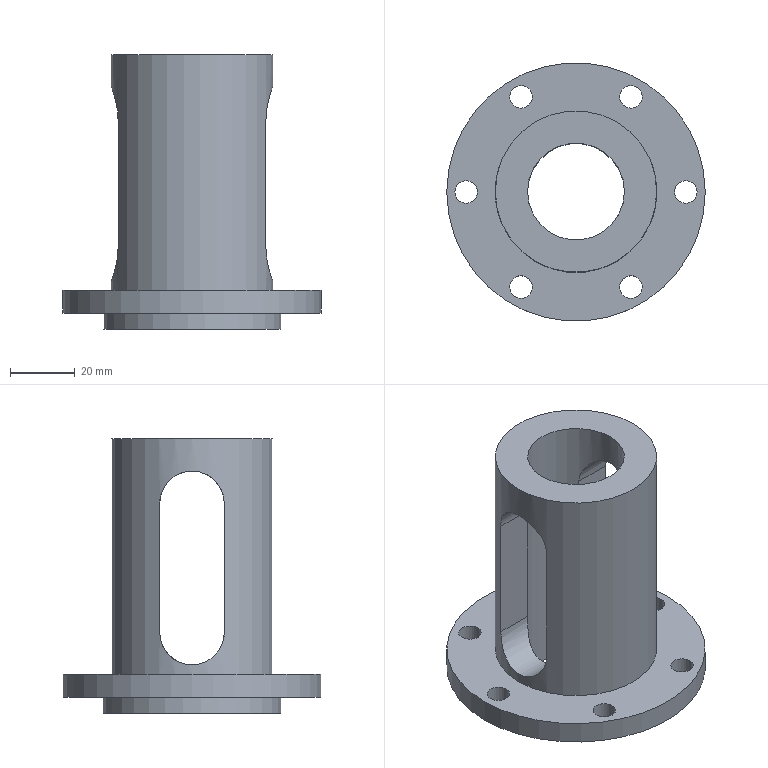NC program | NX | posted with a generic post | part box 80 x 80 x 85 mm
Lines 1745 to 1822 of 1822:
(PROFILE_3D , TOOL : D6A45)
N3488 T05 M6
N3490 G54
N3492 G17 G0 G90 X3.449 Y-17.149 B0. C0. S7500 M3
N3494 G43 Z30. H5
N3496 Z-14.007
N3498 G94 G1 X2.835 Y-16.885 Z-14.186 F1250.
N3500 X1.695 Y-16.572 Z-14.503
N3502 X0.517 Y-16.419 Z-14.822
N3504 X-0.673 Y-16.43 Z-15.14
N3506 X-1.873 Y-16.609 Z-15.466
N3508 X-3.029 Y-16.951 Z-15.788
N3510 X-4.116 Y-17.449 Z-16.109
N3512 X-5.122 Y-18.094 Z-16.429
N3514 X-6.029 Y-18.871 Z-16.749
N3516 X-6.826 Y-19.772 Z-17.071
N3518 X-7.344 Y-20.531 Z-17.318
N3520 X-7.786 Y-21.354 Z-17.568
N3522 X-8.137 Y-22.223 Z-17.819
N3524 X-8.392 Y-23.126 Z-18.07
N3526 X-8.546 Y-24.056 Z-18.323
N3528 X-8.6 Y-25.038 Z-18.587
N3530 Y-64.956 Z-18.557
N3532 X-8.53 Y-66.077 Z-18.556
N3534 X-8.33 Y-67.133 Z-18.46
N3536 X-8.001 Y-68.149 Z-18.278
N3538 X-7.548 Y-69.115 Z-18.095
N3540 X-6.982 Y-70.016 Z-17.857
N3542 X-6.312 Y-70.838 Z-17.62
N3544 X-5.547 Y-71.568 Z-17.383
N3546 X-4.695 Y-72.202 Z-17.146
N3548 X-3.771 Y-72.728 Z-16.908
N3550 X-2.788 Y-73.135 Z-16.75
N3552 X-1.755 Y-73.417 Z-16.591
N3554 X-0.694 Y-73.569 Z-16.518
N3556 X0.503 Y-73.582 Z-16.508
N3558 X1.683 Y-73.431 Z-16.575
N3560 X2.825 Y-73.118 Z-16.747
N3562 X3.913 Y-72.652 Z-16.919
N3564 X4.924 Y-72.046 Z-17.178
N3566 X5.837 Y-71.311 Z-17.436
N3568 X6.641 Y-70.459 Z-17.694
N3570 X7.324 Y-69.502 Z-17.953
N3572 X7.872 Y-68.46 Z-18.212
N3574 X8.271 Y-67.352 Z-18.413
N3576 X8.515 Y-66.19 Z-18.539
N3578 X8.6 Y-64.952 Z-18.586
N3580 Y-25.048
N3582 X8.515 Y-23.811 Z-18.549
N3584 X8.272 Y-22.65 Z-18.434
N3586 X7.873 Y-21.543 Z-18.216
N3588 X7.326 Y-20.501 Z-17.998
N3590 X6.644 Y-19.545 Z-17.736
N3592 X5.841 Y-18.692 Z-17.474
N3594 X4.93 Y-17.958 Z-17.212
N3596 X3.921 Y-17.352 Z-16.949
N3598 X2.835 Y-16.885 Z-16.77
N3600 X1.695 Y-16.572 Z-16.59
N3602 X0.517 Y-16.419 Z-16.513
N3604 X-0.673 Y-16.43 Z-16.512
N3606 X-1.873 Y-16.609 Z-16.588
N3608 X-3.029 Y-16.951 Z-16.737
N3610 X-4.116 Y-17.449 Z-16.978
N3612 X-5.122 Y-18.094 Z-17.218
N3614 X-6.029 Y-18.871 Z-17.488
N3616 X-6.826 Y-19.772 Z-17.76
N3618 X-7.344 Y-20.531 Z-17.967
N3620 X-7.786 Y-21.354 Z-18.179
N3622 X-8.137 Y-22.223 Z-18.327
N3624 X-8.392 Y-23.126 Z-18.475
N3626 X-8.546 Y-24.056 Z-18.53
N3628 X-8.6 Y-25.038 Z-18.587
N3630 Z-17.587
N3632 G0 Z30.
N3634 M5
N3636 M2